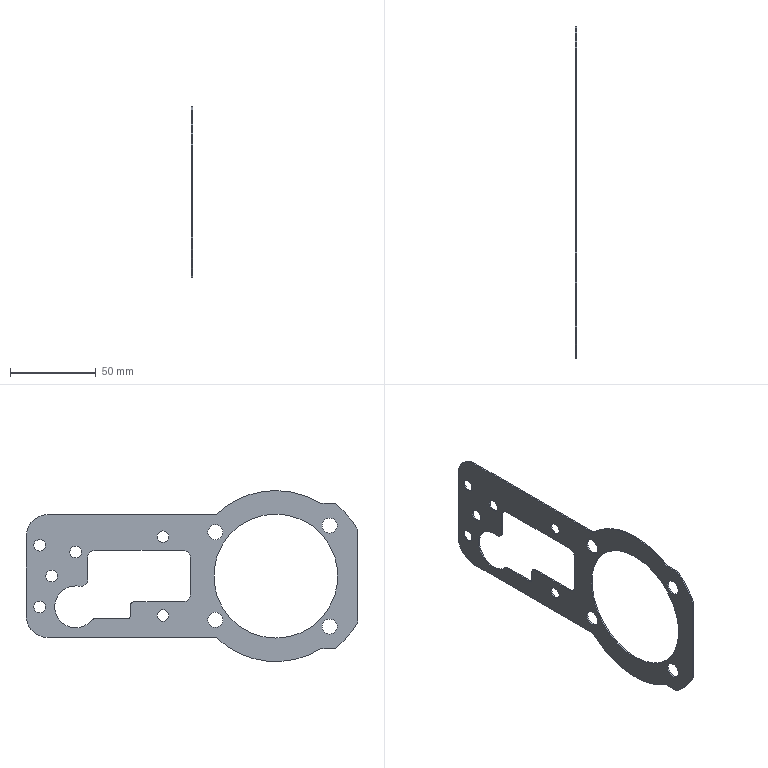Part | SolidWorks | features BaseBody 1 | 1 solid | 53 faces | box 0.8 x 194 x 100 mm | volume 6590 mm3 | cylinder 39 | plane 14 | commonest cylinder face diameters 6.8 x12 8.8 x8 8 x4 4 x3 24.5 x3 100 x3